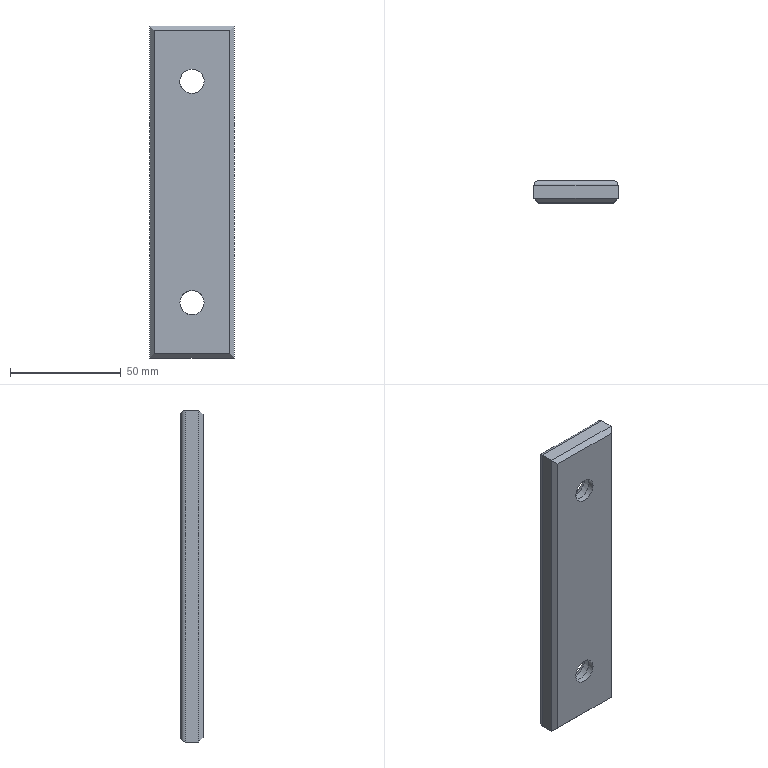Part | NX | features MAIN_BODY 2 | 1 solid | 22 faces | box 38 x 10 x 150 mm | volume 51815 mm3 | plane 12 | cylinder 8 | torus 2 | commonest cylinder face diameters 4 x4 11 x2 17.5 x2
STEP:
#1=CARTESIAN_POINT('',(39.,-393.,-57.));
#2=VERTEX_POINT('',#1);
#3=CARTESIAN_POINT('',(39.,-393.,-203.));
#4=VERTEX_POINT('',#3);
#5=CARTESIAN_POINT('',(39.,-393.,-205.));
#6=DIRECTION('',(0.,0.,1.));
#7=VECTOR('',#6,1000.);
#8=LINE('',#5,#7);
#9=EDGE_CURVE('',#2,#4,#8,.F.);
#10=ORIENTED_EDGE('',*,*,#9,.F.);
#11=CARTESIAN_POINT('',(73.,-393.,-57.));
#12=VERTEX_POINT('',#11);
#13=CARTESIAN_POINT('',(37.,-393.,-57.));
#14=DIRECTION('',(1.,0.,0.));
#15=VECTOR('',#14,1000.);
#16=LINE('',#13,#15);
#17=EDGE_CURVE('',#12,#2,#16,.F.);
#18=ORIENTED_EDGE('',*,*,#17,.F.);
#19=CARTESIAN_POINT('',(73.,-393.,-203.));
#20=VERTEX_POINT('',#19);
#21=CARTESIAN_POINT('',(73.,-393.,-205.));
#22=DIRECTION('',(0.,0.,-1.));
#23=VECTOR('',#22,1000.);
#24=LINE('',#21,#23);
#25=EDGE_CURVE('',#20,#12,#24,.F.);
#26=ORIENTED_EDGE('',*,*,#25,.F.);
#27=CARTESIAN_POINT('',(37.,-393.,-203.));
#28=DIRECTION('',(-1.,0.,0.));
#29=VECTOR('',#28,1000.);
#30=LINE('',#27,#29);
#31=EDGE_CURVE('',#4,#20,#30,.F.);
#32=ORIENTED_EDGE('',*,*,#31,.F.);
#33=EDGE_LOOP('',(#10,#18,#26,#32));
#34=FACE_BOUND('',#33,.T.);
#35=CARTESIAN_POINT('',(56.,-393.,-190.75));
#36=VERTEX_POINT('',#35);
#37=CARTESIAN_POINT('',(56.,-393.,-180.));
#38=DIRECTION('',(0.,-1.,0.));
#39=DIRECTION('',(0.,0.,-1.));
#40=AXIS2_PLACEMENT_3D('',#37,#38,#39);
#41=CIRCLE('',#40,10.75);
#42=EDGE_CURVE('',#36,#36,#41,.F.);
#43=ORIENTED_EDGE('',*,*,#42,.F.);
#44=EDGE_LOOP('',(#43));
#45=FACE_BOUND('',#44,.T.);
#46=CARTESIAN_POINT('',(56.,-393.,-90.75));
#47=VERTEX_POINT('',#46);
#48=CARTESIAN_POINT('',(56.,-393.,-80.));
#49=DIRECTION('',(0.,-1.,0.));
#50=DIRECTION('',(0.,0.,-1.));
#51=AXIS2_PLACEMENT_3D('',#48,#49,#50);
#52=CIRCLE('',#51,10.75);
#53=EDGE_CURVE('',#47,#47,#52,.F.);
#54=ORIENTED_EDGE('',*,*,#53,.F.);
#55=EDGE_LOOP('',(#54));
#56=FACE_BOUND('',#55,.T.);
#57=CARTESIAN_POINT('',(37.,-393.,-205.));
#58=DIRECTION('',(0.,1.,0.));
#59=DIRECTION('',(0.,0.,-1.));
#60=AXIS2_PLACEMENT_3D('',#57,#58,#59);
#61=PLANE('',#60);
#62=ADVANCED_FACE('',(#34,#45,#56),#61,.T.);
#63=CARTESIAN_POINT('',(61.5,-403.,-180.));
#64=VERTEX_POINT('',#63);
#65=CARTESIAN_POINT('',(56.,-403.,-180.));
#66=DIRECTION('',(0.,-1.,0.));
#67=DIRECTION('',(1.,0.,0.));
#68=AXIS2_PLACEMENT_3D('',#65,#66,#67);
#69=CIRCLE('',#68,5.5);
#70=EDGE_CURVE('',#64,#64,#69,.T.);
#71=ORIENTED_EDGE('',*,*,#70,.T.);
#72=EDGE_LOOP('',(#71));
#73=FACE_BOUND('',#72,.T.);
#74=CARTESIAN_POINT('',(56.,-400.3,-185.5));
#75=VERTEX_POINT('',#74);
#76=CARTESIAN_POINT('',(56.,-400.3,-180.));
#77=DIRECTION('',(0.,-1.,0.));
#78=DIRECTION('',(0.,0.,-1.));
#79=AXIS2_PLACEMENT_3D('',#76,#77,#78);
#80=CIRCLE('',#79,5.5);
#81=EDGE_CURVE('',#75,#75,#80,.T.);
#82=ORIENTED_EDGE('',*,*,#81,.F.);
#83=EDGE_LOOP('',(#82));
#84=FACE_BOUND('',#83,.T.);
#85=CARTESIAN_POINT('',(56.,-383.,-180.));
#86=DIRECTION('',(0.,-1.,0.));
#87=DIRECTION('',(0.,0.,1.));
#88=AXIS2_PLACEMENT_3D('',#85,#86,#87);
#89=CYLINDRICAL_SURFACE('',#88,5.5);
#90=ADVANCED_FACE('',(#73,#84),#89,.F.);
#91=CARTESIAN_POINT('',(73.,-403.,-57.));
#92=VERTEX_POINT('',#91);
#93=CARTESIAN_POINT('',(73.,-403.,-203.));
#94=VERTEX_POINT('',#93);
#95=CARTESIAN_POINT('',(73.,-403.,-205.));
#96=DIRECTION('',(0.,0.,-1.));
#97=VECTOR('',#96,1000.);
#98=LINE('',#95,#97);
#99=EDGE_CURVE('',#92,#94,#98,.T.);
#100=ORIENTED_EDGE('',*,*,#99,.F.);
#101=CARTESIAN_POINT('',(39.,-403.,-57.));
#102=VERTEX_POINT('',#101);
#103=CARTESIAN_POINT('',(75.,-403.,-57.));
#104=DIRECTION('',(1.,0.,0.));
#105=VECTOR('',#104,1000.);
#106=LINE('',#103,#105);
#107=EDGE_CURVE('',#102,#92,#106,.T.);
#108=ORIENTED_EDGE('',*,*,#107,.F.);
#109=CARTESIAN_POINT('',(39.,-403.,-203.));
#110=VERTEX_POINT('',#109);
#111=CARTESIAN_POINT('',(39.,-403.,-55.));
#112=DIRECTION('',(0.,0.,1.));
#113=VECTOR('',#112,1000.);
#114=LINE('',#111,#113);
#115=EDGE_CURVE('',#110,#102,#114,.T.);
#116=ORIENTED_EDGE('',*,*,#115,.F.);
#117=CARTESIAN_POINT('',(37.,-403.,-203.));
#118=DIRECTION('',(-1.,0.,0.));
#119=VECTOR('',#118,1000.);
#120=LINE('',#117,#119);
#121=EDGE_CURVE('',#94,#110,#120,.T.);
#122=ORIENTED_EDGE('',*,*,#121,.F.);
#123=EDGE_LOOP('',(#100,#108,#116,#122));
#124=FACE_BOUND('',#123,.T.);
#125=CARTESIAN_POINT('',(61.5,-403.,-80.));
#126=VERTEX_POINT('',#125);
#127=CARTESIAN_POINT('',(56.,-403.,-80.));
#128=DIRECTION('',(0.,1.,0.));
#129=DIRECTION('',(1.,0.,0.));
#130=AXIS2_PLACEMENT_3D('',#127,#128,#129);
#131=CIRCLE('',#130,5.5);
#132=EDGE_CURVE('',#126,#126,#131,.T.);
#133=ORIENTED_EDGE('',*,*,#132,.T.);
#134=EDGE_LOOP('',(#133));
#135=FACE_BOUND('',#134,.T.);
#136=ORIENTED_EDGE('',*,*,#70,.F.);
#137=EDGE_LOOP('',(#136));
#138=FACE_BOUND('',#137,.T.);
#139=CARTESIAN_POINT('',(37.,-403.,-205.));
#140=DIRECTION('',(0.,1.,0.));
#141=DIRECTION('',(0.,0.,-1.));
#142=AXIS2_PLACEMENT_3D('',#139,#140,#141);
#143=PLANE('',#142);
#144=ADVANCED_FACE('',(#124,#135,#138),#143,.F.);
#145=CARTESIAN_POINT('',(37.,-395.,-55.));
#146=VERTEX_POINT('',#145);
#147=CARTESIAN_POINT('',(37.,-401.,-55.));
#148=VERTEX_POINT('',#147);
#149=CARTESIAN_POINT('',(37.,-393.,-55.));
#150=DIRECTION('',(0.,-1.,0.));
#151=VECTOR('',#150,1000.);
#152=LINE('',#149,#151);
#153=EDGE_CURVE('',#146,#148,#152,.T.);
#154=ORIENTED_EDGE('',*,*,#153,.F.);
#155=CARTESIAN_POINT('',(37.,-395.,-205.));
#156=VERTEX_POINT('',#155);
#157=CARTESIAN_POINT('',(37.,-395.,-205.));
#158=DIRECTION('',(0.,0.,1.));
#159=VECTOR('',#158,1000.);
#160=LINE('',#157,#159);
#161=EDGE_CURVE('',#156,#146,#160,.T.);
#162=ORIENTED_EDGE('',*,*,#161,.F.);
#163=CARTESIAN_POINT('',(37.,-401.,-205.));
#164=VERTEX_POINT('',#163);
#165=CARTESIAN_POINT('',(37.,-393.,-205.));
#166=DIRECTION('',(0.,-1.,0.));
#167=VECTOR('',#166,1000.);
#168=LINE('',#165,#167);
#169=EDGE_CURVE('',#156,#164,#168,.T.);
#170=ORIENTED_EDGE('',*,*,#169,.T.);
#171=CARTESIAN_POINT('',(37.,-401.,-205.));
#172=DIRECTION('',(0.,0.,-1.));
#173=VECTOR('',#172,1000.);
#174=LINE('',#171,#173);
#175=EDGE_CURVE('',#148,#164,#174,.T.);
#176=ORIENTED_EDGE('',*,*,#175,.F.);
#177=EDGE_LOOP('',(#154,#162,#170,#176));
#178=FACE_BOUND('',#177,.T.);
#179=CARTESIAN_POINT('',(37.,-393.,-205.));
#180=DIRECTION('',(-1.,0.,0.));
#181=DIRECTION('',(0.,0.,-1.));
#182=AXIS2_PLACEMENT_3D('',#179,#180,#181);
#183=PLANE('',#182);
#184=ADVANCED_FACE('',(#178),#183,.T.);
#185=CARTESIAN_POINT('',(75.,-395.,-55.));
#186=VERTEX_POINT('',#185);
#187=CARTESIAN_POINT('',(75.,-401.,-55.));
#188=VERTEX_POINT('',#187);
#189=CARTESIAN_POINT('',(75.,-393.,-55.));
#190=DIRECTION('',(0.,-1.,0.));
#191=VECTOR('',#190,1000.);
#192=LINE('',#189,#191);
#193=EDGE_CURVE('',#186,#188,#192,.T.);
#194=ORIENTED_EDGE('',*,*,#193,.F.);
#195=CARTESIAN_POINT('',(37.,-395.,-55.));
#196=DIRECTION('',(1.,0.,0.));
#197=VECTOR('',#196,1000.);
#198=LINE('',#195,#197);
#199=EDGE_CURVE('',#146,#186,#198,.T.);
#200=ORIENTED_EDGE('',*,*,#199,.F.);
#201=ORIENTED_EDGE('',*,*,#153,.T.);
#202=CARTESIAN_POINT('',(37.,-401.,-55.));
#203=DIRECTION('',(-1.,0.,0.));
#204=VECTOR('',#203,1000.);
#205=LINE('',#202,#204);
#206=EDGE_CURVE('',#188,#148,#205,.T.);
#207=ORIENTED_EDGE('',*,*,#206,.F.);
#208=EDGE_LOOP('',(#194,#200,#201,#207));
#209=FACE_BOUND('',#208,.T.);
#210=CARTESIAN_POINT('',(37.,-393.,-55.));
#211=DIRECTION('',(0.,0.,1.));
#212=DIRECTION('',(0.,1.,0.));
#213=AXIS2_PLACEMENT_3D('',#210,#211,#212);
#214=PLANE('',#213);
#215=ADVANCED_FACE('',(#209),#214,.T.);
#216=CARTESIAN_POINT('',(75.,-395.,-205.));
#217=VERTEX_POINT('',#216);
#218=CARTESIAN_POINT('',(75.,-401.,-205.));
#219=VERTEX_POINT('',#218);
#220=CARTESIAN_POINT('',(75.,-393.,-205.));
#221=DIRECTION('',(0.,-1.,0.));
#222=VECTOR('',#221,1000.);
#223=LINE('',#220,#222);
#224=EDGE_CURVE('',#217,#219,#223,.T.);
#225=ORIENTED_EDGE('',*,*,#224,.F.);
#226=CARTESIAN_POINT('',(75.,-395.,-55.));
#227=DIRECTION('',(0.,0.,-1.));
#228=VECTOR('',#227,1000.);
#229=LINE('',#226,#228);
#230=EDGE_CURVE('',#186,#217,#229,.T.);
#231=ORIENTED_EDGE('',*,*,#230,.F.);
#232=ORIENTED_EDGE('',*,*,#193,.T.);
#233=CARTESIAN_POINT('',(75.,-401.,-55.));
#234=DIRECTION('',(0.,0.,1.));
#235=VECTOR('',#234,1000.);
#236=LINE('',#233,#235);
#237=EDGE_CURVE('',#219,#188,#236,.T.);
#238=ORIENTED_EDGE('',*,*,#237,.F.);
#239=EDGE_LOOP('',(#225,#231,#232,#238));
#240=FACE_BOUND('',#239,.T.);
#241=CARTESIAN_POINT('',(75.,-393.,-55.));
#242=DIRECTION('',(1.,0.,0.));
#243=DIRECTION('',(0.,0.,1.));
#244=AXIS2_PLACEMENT_3D('',#241,#242,#243);
#245=PLANE('',#244);
#246=ADVANCED_FACE('',(#240),#245,.T.);
#247=ORIENTED_EDGE('',*,*,#169,.F.);
#248=CARTESIAN_POINT('',(75.,-395.,-205.));
#249=DIRECTION('',(-1.,0.,0.));
#250=VECTOR('',#249,1000.);
#251=LINE('',#248,#250);
#252=EDGE_CURVE('',#217,#156,#251,.T.);
#253=ORIENTED_EDGE('',*,*,#252,.F.);
#254=ORIENTED_EDGE('',*,*,#224,.T.);
#255=CARTESIAN_POINT('',(75.,-401.,-205.));
#256=DIRECTION('',(1.,0.,0.));
#257=VECTOR('',#256,1000.);
#258=LINE('',#255,#257);
#259=EDGE_CURVE('',#164,#219,#258,.T.);
#260=ORIENTED_EDGE('',*,*,#259,.F.);
#261=EDGE_LOOP('',(#247,#253,#254,#260));
#262=FACE_BOUND('',#261,.T.);
#263=CARTESIAN_POINT('',(75.,-393.,-205.));
#264=DIRECTION('',(0.,0.,-1.));
#265=DIRECTION('',(1.,0.,0.));
#266=AXIS2_PLACEMENT_3D('',#263,#264,#265);
#267=PLANE('',#266);
#268=ADVANCED_FACE('',(#262),#267,.T.);
#269=CARTESIAN_POINT('',(56.,-400.3,-74.5));
#270=VERTEX_POINT('',#269);
#271=CARTESIAN_POINT('',(56.,-400.3,-80.));
#272=DIRECTION('',(0.,1.,0.));
#273=DIRECTION('',(0.,0.,1.));
#274=AXIS2_PLACEMENT_3D('',#271,#272,#273);
#275=CIRCLE('',#274,5.5);
#276=EDGE_CURVE('',#270,#270,#275,.F.);
#277=ORIENTED_EDGE('',*,*,#276,.F.);
#278=EDGE_LOOP('',(#277));
#279=FACE_BOUND('',#278,.T.);
#280=ORIENTED_EDGE('',*,*,#132,.F.);
#281=EDGE_LOOP('',(#280));
#282=FACE_BOUND('',#281,.T.);
#283=CARTESIAN_POINT('',(56.,-383.,-80.));
#284=DIRECTION('',(0.,-1.,0.));
#285=DIRECTION('',(0.,0.,1.));
#286=AXIS2_PLACEMENT_3D('',#283,#284,#285);
#287=CYLINDRICAL_SURFACE('',#286,5.5);
#288=ADVANCED_FACE('',(#279,#282),#287,.F.);
#289=CARTESIAN_POINT('',(56.,-395.,-188.75));
#290=VERTEX_POINT('',#289);
#291=CARTESIAN_POINT('',(56.,-395.,-180.));
#292=DIRECTION('',(0.,-1.,0.));
#293=DIRECTION('',(0.,0.,-1.));
#294=AXIS2_PLACEMENT_3D('',#291,#292,#293);
#295=CIRCLE('',#294,8.75);
#296=EDGE_CURVE('',#290,#290,#295,.T.);
#297=ORIENTED_EDGE('',*,*,#296,.F.);
#298=EDGE_LOOP('',(#297));
#299=FACE_BOUND('',#298,.T.);
#300=CARTESIAN_POINT('',(64.75,-400.3,-180.));
#301=VERTEX_POINT('',#300);
#302=CARTESIAN_POINT('',(56.,-400.3,-180.));
#303=DIRECTION('',(0.,-1.,0.));
#304=DIRECTION('',(1.,0.,0.));
#305=AXIS2_PLACEMENT_3D('',#302,#303,#304);
#306=CIRCLE('',#305,8.75);
#307=EDGE_CURVE('',#301,#301,#306,.T.);
#308=ORIENTED_EDGE('',*,*,#307,.T.);
#309=EDGE_LOOP('',(#308));
#310=FACE_BOUND('',#309,.T.);
#311=CARTESIAN_POINT('',(56.,-373.,-180.));
#312=DIRECTION('',(0.,-1.,0.));
#313=DIRECTION('',(0.,0.,1.));
#314=AXIS2_PLACEMENT_3D('',#311,#312,#313);
#315=CYLINDRICAL_SURFACE('',#314,8.75);
#316=ADVANCED_FACE('',(#299,#310),#315,.F.);
#317=ORIENTED_EDGE('',*,*,#81,.T.);
#318=EDGE_LOOP('',(#317));
#319=FACE_BOUND('',#318,.T.);
#320=ORIENTED_EDGE('',*,*,#307,.F.);
#321=EDGE_LOOP('',(#320));
#322=FACE_BOUND('',#321,.T.);
#323=CARTESIAN_POINT('',(56.,-400.3,-180.));
#324=DIRECTION('',(0.,1.,0.));
#325=DIRECTION('',(0.,0.,-1.));
#326=AXIS2_PLACEMENT_3D('',#323,#324,#325);
#327=PLANE('',#326);
#328=ADVANCED_FACE('',(#319,#322),#327,.T.);
#329=CARTESIAN_POINT('',(64.75,-400.3,-80.));
#330=VERTEX_POINT('',#329);
#331=CARTESIAN_POINT('',(56.,-400.3,-80.));
#332=DIRECTION('',(0.,1.,0.));
#333=DIRECTION('',(1.,0.,0.));
#334=AXIS2_PLACEMENT_3D('',#331,#332,#333);
#335=CIRCLE('',#334,8.75);
#336=EDGE_CURVE('',#330,#330,#335,.T.);
#337=ORIENTED_EDGE('',*,*,#336,.T.);
#338=EDGE_LOOP('',(#337));
#339=FACE_BOUND('',#338,.T.);
#340=ORIENTED_EDGE('',*,*,#276,.T.);
#341=EDGE_LOOP('',(#340));
#342=FACE_BOUND('',#341,.T.);
#343=CARTESIAN_POINT('',(56.,-400.3,-80.));
#344=DIRECTION('',(0.,-1.,0.));
#345=DIRECTION('',(0.,0.,1.));
#346=AXIS2_PLACEMENT_3D('',#343,#344,#345);
#347=PLANE('',#346);
#348=ADVANCED_FACE('',(#339,#342),#347,.F.);
#349=CARTESIAN_POINT('',(56.,-395.,-88.75));
#350=VERTEX_POINT('',#349);
#351=CARTESIAN_POINT('',(56.,-395.,-80.));
#352=DIRECTION('',(0.,-1.,0.));
#353=DIRECTION('',(0.,0.,-1.));
#354=AXIS2_PLACEMENT_3D('',#351,#352,#353);
#355=CIRCLE('',#354,8.75);
#356=EDGE_CURVE('',#350,#350,#355,.T.);
#357=ORIENTED_EDGE('',*,*,#356,.F.);
#358=EDGE_LOOP('',(#357));
#359=FACE_BOUND('',#358,.T.);
#360=ORIENTED_EDGE('',*,*,#336,.F.);
#361=EDGE_LOOP('',(#360));
#362=FACE_BOUND('',#361,.T.);
#363=CARTESIAN_POINT('',(56.,-373.,-80.));
#364=DIRECTION('',(0.,-1.,0.));
#365=DIRECTION('',(0.,0.,1.));
#366=AXIS2_PLACEMENT_3D('',#363,#364,#365);
#367=CYLINDRICAL_SURFACE('',#366,8.75);
#368=ADVANCED_FACE('',(#359,#362),#367,.F.);
#369=CARTESIAN_POINT('',(39.,-395.,-57.));
#370=DIRECTION('',(-0.7071,0.,-0.7071));
#371=DIRECTION('',(0.7071,0.,-0.7071));
#372=AXIS2_PLACEMENT_3D('',#369,#370,#371);
#373=ELLIPSE('',#372,2.828,2.);
#374=EDGE_CURVE('',#2,#146,#373,.F.);
#375=ORIENTED_EDGE('',*,*,#374,.T.);
#376=ORIENTED_EDGE('',*,*,#199,.T.);
#377=CARTESIAN_POINT('',(73.,-395.,-57.));
#378=DIRECTION('',(-0.7071,0.,0.7071));
#379=DIRECTION('',(0.7071,0.,0.7071));
#380=AXIS2_PLACEMENT_3D('',#377,#378,#379);
#381=ELLIPSE('',#380,2.828,2.);
#382=EDGE_CURVE('',#186,#12,#381,.T.);
#383=ORIENTED_EDGE('',*,*,#382,.T.);
#384=ORIENTED_EDGE('',*,*,#17,.T.);
#385=EDGE_LOOP('',(#375,#376,#383,#384));
#386=FACE_BOUND('',#385,.T.);
#387=CARTESIAN_POINT('',(37.,-395.,-57.));
#388=DIRECTION('',(1.,0.,0.));
#389=DIRECTION('',(0.,0.,1.));
#390=AXIS2_PLACEMENT_3D('',#387,#388,#389);
#391=CYLINDRICAL_SURFACE('',#390,2.);
#392=ADVANCED_FACE('',(#386),#391,.T.);
#393=ORIENTED_EDGE('',*,*,#382,.F.);
#394=ORIENTED_EDGE('',*,*,#230,.T.);
#395=CARTESIAN_POINT('',(73.,-395.,-203.));
#396=DIRECTION('',(0.7071,0.,0.7071));
#397=DIRECTION('',(0.7071,0.,-0.7071));
#398=AXIS2_PLACEMENT_3D('',#395,#396,#397);
#399=ELLIPSE('',#398,2.828,2.);
#400=EDGE_CURVE('',#217,#20,#399,.T.);
#401=ORIENTED_EDGE('',*,*,#400,.T.);
#402=ORIENTED_EDGE('',*,*,#25,.T.);
#403=EDGE_LOOP('',(#393,#394,#401,#402));
#404=FACE_BOUND('',#403,.T.);
#405=CARTESIAN_POINT('',(73.,-395.,-55.));
#406=DIRECTION('',(0.,0.,-1.));
#407=DIRECTION('',(0.,-1.,0.));
#408=AXIS2_PLACEMENT_3D('',#405,#406,#407);
#409=CYLINDRICAL_SURFACE('',#408,2.);
#410=ADVANCED_FACE('',(#404),#409,.T.);
#411=ORIENTED_EDGE('',*,*,#374,.F.);
#412=ORIENTED_EDGE('',*,*,#9,.T.);
#413=CARTESIAN_POINT('',(39.,-395.,-203.));
#414=DIRECTION('',(0.7071,0.,-0.7071));
#415=DIRECTION('',(0.7071,0.,0.7071));
#416=AXIS2_PLACEMENT_3D('',#413,#414,#415);
#417=ELLIPSE('',#416,2.828,2.);
#418=EDGE_CURVE('',#4,#156,#417,.F.);
#419=ORIENTED_EDGE('',*,*,#418,.T.);
#420=ORIENTED_EDGE('',*,*,#161,.T.);
#421=EDGE_LOOP('',(#411,#412,#419,#420));
#422=FACE_BOUND('',#421,.T.);
#423=CARTESIAN_POINT('',(39.,-395.,-205.));
#424=DIRECTION('',(0.,0.,1.));
#425=DIRECTION('',(-1.,0.,0.));
#426=AXIS2_PLACEMENT_3D('',#423,#424,#425);
#427=CYLINDRICAL_SURFACE('',#426,2.);
#428=ADVANCED_FACE('',(#422),#427,.T.);
#429=ORIENTED_EDGE('',*,*,#400,.F.);
#430=ORIENTED_EDGE('',*,*,#252,.T.);
#431=ORIENTED_EDGE('',*,*,#418,.F.);
#432=ORIENTED_EDGE('',*,*,#31,.T.);
#433=EDGE_LOOP('',(#429,#430,#431,#432));
#434=FACE_BOUND('',#433,.T.);
#435=CARTESIAN_POINT('',(75.,-395.,-203.));
#436=DIRECTION('',(-1.,0.,0.));
#437=DIRECTION('',(0.,0.,-1.));
#438=AXIS2_PLACEMENT_3D('',#435,#436,#437);
#439=CYLINDRICAL_SURFACE('',#438,2.);
#440=ADVANCED_FACE('',(#434),#439,.T.);
#441=ORIENTED_EDGE('',*,*,#296,.T.);
#442=EDGE_LOOP('',(#441));
#443=FACE_BOUND('',#442,.T.);
#444=ORIENTED_EDGE('',*,*,#42,.T.);
#445=EDGE_LOOP('',(#444));
#446=FACE_BOUND('',#445,.T.);
#447=CARTESIAN_POINT('',(56.,-395.,-180.));
#448=DIRECTION('',(0.,1.,0.));
#449=DIRECTION('',(0.,0.,-1.));
#450=AXIS2_PLACEMENT_3D('',#447,#448,#449);
#451=TOROIDAL_SURFACE('',#450,10.75,2.);
#452=ADVANCED_FACE('',(#443,#446),#451,.T.);
#453=ORIENTED_EDGE('',*,*,#53,.T.);
#454=EDGE_LOOP('',(#453));
#455=FACE_BOUND('',#454,.T.);
#456=ORIENTED_EDGE('',*,*,#356,.T.);
#457=EDGE_LOOP('',(#456));
#458=FACE_BOUND('',#457,.T.);
#459=CARTESIAN_POINT('',(56.,-395.,-80.));
#460=DIRECTION('',(0.,1.,0.));
#461=DIRECTION('',(0.,0.,-1.));
#462=AXIS2_PLACEMENT_3D('',#459,#460,#461);
#463=TOROIDAL_SURFACE('',#462,10.75,2.);
#464=ADVANCED_FACE('',(#455,#458),#463,.T.);
#465=CARTESIAN_POINT('',(38.333,-402.333,-56.333));
#466=DIRECTION('',(-0.5774,0.5774,0.5774));
#467=VECTOR('',#466,1000.);
#468=LINE('',#465,#467);
#469=EDGE_CURVE('',#148,#102,#468,.F.);
#470=ORIENTED_EDGE('',*,*,#469,.T.);
#471=ORIENTED_EDGE('',*,*,#107,.T.);
#472=CARTESIAN_POINT('',(23.667,-452.333,-106.333));
#473=DIRECTION('',(0.5774,0.5774,0.5774));
#474=VECTOR('',#473,1000.);
#475=LINE('',#472,#474);
#476=EDGE_CURVE('',#92,#188,#475,.T.);
#477=ORIENTED_EDGE('',*,*,#476,.T.);
#478=ORIENTED_EDGE('',*,*,#206,.T.);
#479=EDGE_LOOP('',(#470,#471,#477,#478));
#480=FACE_BOUND('',#479,.T.);
#481=CARTESIAN_POINT('',(37.,-403.,-57.));
#482=DIRECTION('',(0.,-0.7071,0.7071));
#483=DIRECTION('',(0.,0.7071,0.7071));
#484=AXIS2_PLACEMENT_3D('',#481,#482,#483);
#485=PLANE('',#484);
#486=ADVANCED_FACE('',(#480),#485,.T.);
#487=ORIENTED_EDGE('',*,*,#476,.F.);
#488=ORIENTED_EDGE('',*,*,#99,.T.);
#489=CARTESIAN_POINT('',(73.667,-402.333,-203.667));
#490=DIRECTION('',(-0.5774,-0.5774,0.5774));
#491=VECTOR('',#490,1000.);
#492=LINE('',#489,#491);
#493=EDGE_CURVE('',#94,#219,#492,.F.);
#494=ORIENTED_EDGE('',*,*,#493,.T.);
#495=ORIENTED_EDGE('',*,*,#237,.T.);
#496=EDGE_LOOP('',(#487,#488,#494,#495));
#497=FACE_BOUND('',#496,.T.);
#498=CARTESIAN_POINT('',(73.,-403.,-205.));
#499=DIRECTION('',(0.7071,-0.7071,0.));
#500=DIRECTION('',(-0.7071,-0.7071,0.));
#501=AXIS2_PLACEMENT_3D('',#498,#499,#500);
#502=PLANE('',#501);
#503=ADVANCED_FACE('',(#497),#502,.T.);
#504=ORIENTED_EDGE('',*,*,#469,.F.);
#505=ORIENTED_EDGE('',*,*,#175,.T.);
#506=CARTESIAN_POINT('',(38.333,-402.333,-203.667));
#507=DIRECTION('',(-0.5774,0.5774,-0.5774));
#508=VECTOR('',#507,1000.);
#509=LINE('',#506,#508);
#510=EDGE_CURVE('',#164,#110,#509,.F.);
#511=ORIENTED_EDGE('',*,*,#510,.T.);
#512=ORIENTED_EDGE('',*,*,#115,.T.);
#513=EDGE_LOOP('',(#504,#505,#511,#512));
#514=FACE_BOUND('',#513,.T.);
#515=CARTESIAN_POINT('',(39.,-403.,-205.));
#516=DIRECTION('',(-0.7071,-0.7071,0.));
#517=DIRECTION('',(-0.7071,0.7071,0.));
#518=AXIS2_PLACEMENT_3D('',#515,#516,#517);
#519=PLANE('',#518);
#520=ADVANCED_FACE('',(#514),#519,.T.);
#521=ORIENTED_EDGE('',*,*,#493,.F.);
#522=ORIENTED_EDGE('',*,*,#121,.T.);
#523=ORIENTED_EDGE('',*,*,#510,.F.);
#524=ORIENTED_EDGE('',*,*,#259,.T.);
#525=EDGE_LOOP('',(#521,#522,#523,#524));
#526=FACE_BOUND('',#525,.T.);
#527=CARTESIAN_POINT('',(37.,-403.,-203.));
#528=DIRECTION('',(0.,-0.7071,-0.7071));
#529=DIRECTION('',(0.,-0.7071,0.7071));
#530=AXIS2_PLACEMENT_3D('',#527,#528,#529);
#531=PLANE('',#530);
#532=ADVANCED_FACE('',(#526),#531,.T.);
#533=CLOSED_SHELL('',(#62,#90,#144,#184,#215,#246,#268,#288,#316,#328,#348,#368,#392,#410,#428,#440,#452,#464,#486,#503,#520,#532));
#534=MANIFOLD_SOLID_BREP('',#533);
#535=(LENGTH_UNIT()NAMED_UNIT(*)SI_UNIT(.MILLI.,.METRE.));
#536=UNCERTAINTY_MEASURE_WITH_UNIT(LENGTH_MEASURE(0.00001),#535,'','');
#537=(NAMED_UNIT(*)PLANE_ANGLE_UNIT()SI_UNIT($,.RADIAN.));
#538=(NAMED_UNIT(*)SI_UNIT($,.STERADIAN.)SOLID_ANGLE_UNIT());
#539=(GEOMETRIC_REPRESENTATION_CONTEXT(3)GLOBAL_UNCERTAINTY_ASSIGNED_CONTEXT((#536))GLOBAL_UNIT_ASSIGNED_CONTEXT((#535,#537,#538))REPRESENTATION_CONTEXT('',''));
#540=ADVANCED_BREP_SHAPE_REPRESENTATION('',(#534),#539);